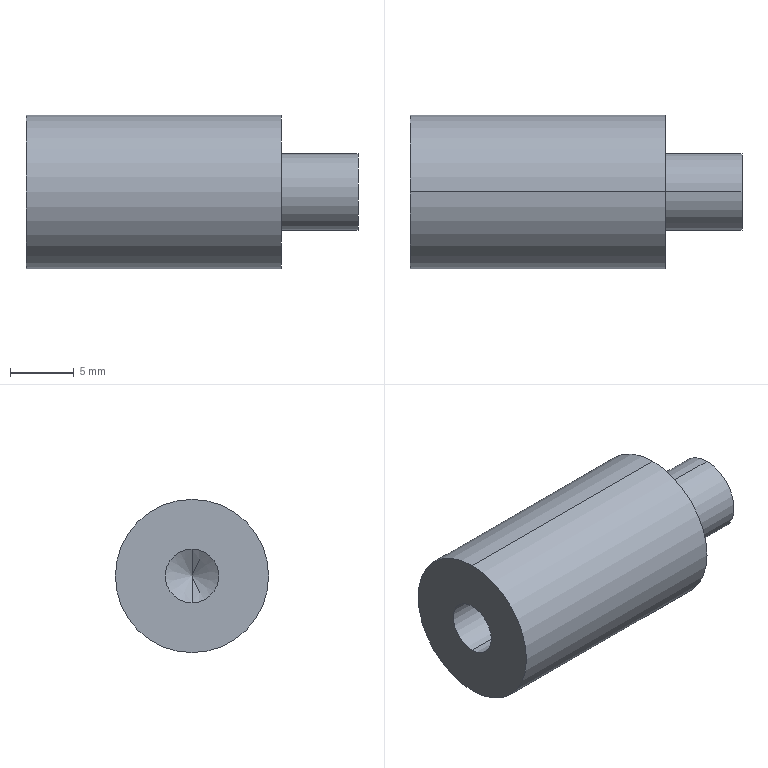Part | STEP file | Tension support column | 1 solid | 15 faces | box 26 x 12 x 12 mm | volume 2216 mm3 | cylinder 8 | cone 4 | plane 3 | commonest cylinder face diameters 2.5 x2 4.2 x2 6 x2 12 x2
STEP:
#1=CARTESIAN_POINT('',(12.4,0.,-2.1));
#2=VERTEX_POINT('',#1);
#3=CARTESIAN_POINT('',(12.4,0.,2.1));
#4=VERTEX_POINT('',#3);
#5=CARTESIAN_POINT('',(12.4,0.,0.));
#6=DIRECTION('',(-1.,0.,0.));
#7=DIRECTION('',(0.,0.,1.));
#8=AXIS2_PLACEMENT_3D('',#5,#6,#7);
#9=CIRCLE('',#8,2.1);
#10=EDGE_CURVE('',#2,#4,#9,.T.);
#11=ORIENTED_EDGE('',*,*,#10,.F.);
#12=CARTESIAN_POINT('',(0.,0.,-2.1));
#13=VERTEX_POINT('',#12);
#14=CARTESIAN_POINT('',(0.,0.,-2.1));
#15=DIRECTION('',(-1.,0.,0.));
#16=VECTOR('',#15,1000.);
#17=LINE('',#14,#16);
#18=EDGE_CURVE('',#2,#13,#17,.T.);
#19=ORIENTED_EDGE('',*,*,#18,.T.);
#20=CARTESIAN_POINT('',(0.,0.,2.1));
#21=VERTEX_POINT('',#20);
#22=CARTESIAN_POINT('',(0.,0.,0.));
#23=DIRECTION('',(-1.,0.,0.));
#24=DIRECTION('',(0.,0.,1.));
#25=AXIS2_PLACEMENT_3D('',#22,#23,#24);
#26=CIRCLE('',#25,2.1);
#27=EDGE_CURVE('',#13,#21,#26,.T.);
#28=ORIENTED_EDGE('',*,*,#27,.T.);
#29=CARTESIAN_POINT('',(0.,0.,2.1));
#30=DIRECTION('',(-1.,0.,0.));
#31=VECTOR('',#30,1000.);
#32=LINE('',#29,#31);
#33=EDGE_CURVE('',#4,#21,#32,.T.);
#34=ORIENTED_EDGE('',*,*,#33,.F.);
#35=EDGE_LOOP('',(#11,#19,#28,#34));
#36=FACE_OUTER_BOUND('',#35,.T.);
#37=CARTESIAN_POINT('',(0.,0.,0.));
#38=DIRECTION('',(-1.,0.,0.));
#39=DIRECTION('',(0.,0.,1.));
#40=AXIS2_PLACEMENT_3D('',#37,#38,#39);
#41=CYLINDRICAL_SURFACE('',#40,2.1);
#42=ADVANCED_FACE('',(#36),#41,.F.);
#43=CARTESIAN_POINT('',(13.662,0.,0.));
#44=VERTEX_POINT('',#43);
#45=CARTESIAN_POINT('',(12.4,0.,2.1));
#46=DIRECTION('',(-0.515,0.,0.8572));
#47=VECTOR('',#46,1000.);
#48=LINE('',#45,#47);
#49=EDGE_CURVE('',#44,#4,#48,.T.);
#50=ORIENTED_EDGE('',*,*,#49,.F.);
#51=CARTESIAN_POINT('',(12.4,0.,-2.1));
#52=DIRECTION('',(-0.515,0.,-0.8572));
#53=VECTOR('',#52,1000.);
#54=LINE('',#51,#53);
#55=EDGE_CURVE('',#44,#2,#54,.T.);
#56=ORIENTED_EDGE('',*,*,#55,.T.);
#57=ORIENTED_EDGE('',*,*,#10,.T.);
#58=EDGE_LOOP('',(#50,#56,#57));
#59=FACE_OUTER_BOUND('',#58,.T.);
#60=CARTESIAN_POINT('',(12.4,0.,0.));
#61=DIRECTION('',(-1.,0.,0.));
#62=DIRECTION('',(0.,0.,1.));
#63=AXIS2_PLACEMENT_3D('',#60,#61,#62);
#64=CONICAL_SURFACE('',#63,2.1,1.03);
#65=ADVANCED_FACE('',(#59),#64,.F.);
#66=CARTESIAN_POINT('',(18.5,0.,1.25));
#67=VERTEX_POINT('',#66);
#68=CARTESIAN_POINT('',(18.5,0.,-1.25));
#69=VERTEX_POINT('',#68);
#70=CARTESIAN_POINT('',(18.5,0.,0.));
#71=DIRECTION('',(1.,0.,0.));
#72=DIRECTION('',(0.,0.,-1.));
#73=AXIS2_PLACEMENT_3D('',#70,#71,#72);
#74=CIRCLE('',#73,1.25);
#75=EDGE_CURVE('',#67,#69,#74,.T.);
#76=ORIENTED_EDGE('',*,*,#75,.F.);
#77=CARTESIAN_POINT('',(26.,0.,1.25));
#78=VERTEX_POINT('',#77);
#79=CARTESIAN_POINT('',(26.,0.,1.25));
#80=DIRECTION('',(1.,0.,0.));
#81=VECTOR('',#80,1000.);
#82=LINE('',#79,#81);
#83=EDGE_CURVE('',#67,#78,#82,.T.);
#84=ORIENTED_EDGE('',*,*,#83,.T.);
#85=CARTESIAN_POINT('',(26.,0.,-1.25));
#86=VERTEX_POINT('',#85);
#87=CARTESIAN_POINT('',(26.,0.,0.));
#88=DIRECTION('',(1.,0.,0.));
#89=DIRECTION('',(0.,0.,-1.));
#90=AXIS2_PLACEMENT_3D('',#87,#88,#89);
#91=CIRCLE('',#90,1.25);
#92=EDGE_CURVE('',#78,#86,#91,.T.);
#93=ORIENTED_EDGE('',*,*,#92,.T.);
#94=CARTESIAN_POINT('',(26.,0.,-1.25));
#95=DIRECTION('',(1.,0.,0.));
#96=VECTOR('',#95,1000.);
#97=LINE('',#94,#96);
#98=EDGE_CURVE('',#69,#86,#97,.T.);
#99=ORIENTED_EDGE('',*,*,#98,.F.);
#100=EDGE_LOOP('',(#76,#84,#93,#99));
#101=FACE_OUTER_BOUND('',#100,.T.);
#102=CARTESIAN_POINT('',(26.,0.,0.));
#103=DIRECTION('',(1.,0.,0.));
#104=DIRECTION('',(0.,0.,-1.));
#105=AXIS2_PLACEMENT_3D('',#102,#103,#104);
#106=CYLINDRICAL_SURFACE('',#105,1.25);
#107=ADVANCED_FACE('',(#101),#106,.F.);
#108=CARTESIAN_POINT('',(17.749,0.,0.));
#109=VERTEX_POINT('',#108);
#110=CARTESIAN_POINT('',(18.5,0.,-1.25));
#111=DIRECTION('',(0.515,0.,-0.8572));
#112=VECTOR('',#111,1000.);
#113=LINE('',#110,#112);
#114=EDGE_CURVE('',#109,#69,#113,.T.);
#115=ORIENTED_EDGE('',*,*,#114,.F.);
#116=CARTESIAN_POINT('',(18.5,0.,1.25));
#117=DIRECTION('',(0.515,0.,0.8572));
#118=VECTOR('',#117,1000.);
#119=LINE('',#116,#118);
#120=EDGE_CURVE('',#109,#67,#119,.T.);
#121=ORIENTED_EDGE('',*,*,#120,.T.);
#122=ORIENTED_EDGE('',*,*,#75,.T.);
#123=EDGE_LOOP('',(#115,#121,#122));
#124=FACE_OUTER_BOUND('',#123,.T.);
#125=CARTESIAN_POINT('',(18.5,0.,0.));
#126=DIRECTION('',(1.,0.,0.));
#127=DIRECTION('',(0.,0.,-1.));
#128=AXIS2_PLACEMENT_3D('',#125,#126,#127);
#129=CONICAL_SURFACE('',#128,1.25,1.03);
#130=ADVANCED_FACE('',(#124),#129,.F.);
#131=CARTESIAN_POINT('',(20.,0.,-3.));
#132=VERTEX_POINT('',#131);
#133=CARTESIAN_POINT('',(20.,0.,3.));
#134=VERTEX_POINT('',#133);
#135=CARTESIAN_POINT('',(20.,0.,0.));
#136=DIRECTION('',(1.,0.,0.));
#137=DIRECTION('',(0.,0.,-1.));
#138=AXIS2_PLACEMENT_3D('',#135,#136,#137);
#139=CIRCLE('',#138,3.);
#140=EDGE_CURVE('',#132,#134,#139,.T.);
#141=ORIENTED_EDGE('',*,*,#140,.T.);
#142=CARTESIAN_POINT('',(26.,0.,3.));
#143=VERTEX_POINT('',#142);
#144=CARTESIAN_POINT('',(0.,0.,3.));
#145=DIRECTION('',(1.,0.,0.));
#146=VECTOR('',#145,1000.);
#147=LINE('',#144,#146);
#148=EDGE_CURVE('',#134,#143,#147,.T.);
#149=ORIENTED_EDGE('',*,*,#148,.T.);
#150=CARTESIAN_POINT('',(26.,0.,-3.));
#151=VERTEX_POINT('',#150);
#152=CARTESIAN_POINT('',(26.,0.,0.));
#153=DIRECTION('',(1.,0.,0.));
#154=DIRECTION('',(0.,0.,-1.));
#155=AXIS2_PLACEMENT_3D('',#152,#153,#154);
#156=CIRCLE('',#155,3.);
#157=EDGE_CURVE('',#151,#143,#156,.T.);
#158=ORIENTED_EDGE('',*,*,#157,.F.);
#159=CARTESIAN_POINT('',(0.,0.,-3.));
#160=DIRECTION('',(1.,0.,0.));
#161=VECTOR('',#160,1000.);
#162=LINE('',#159,#161);
#163=EDGE_CURVE('',#132,#151,#162,.T.);
#164=ORIENTED_EDGE('',*,*,#163,.F.);
#165=EDGE_LOOP('',(#141,#149,#158,#164));
#166=FACE_OUTER_BOUND('',#165,.T.);
#167=CARTESIAN_POINT('',(0.,0.,0.));
#168=DIRECTION('',(1.,0.,0.));
#169=DIRECTION('',(0.,0.,-1.));
#170=AXIS2_PLACEMENT_3D('',#167,#168,#169);
#171=CYLINDRICAL_SURFACE('',#170,3.);
#172=ADVANCED_FACE('',(#166),#171,.T.);
#173=CARTESIAN_POINT('',(0.,0.,-6.));
#174=VERTEX_POINT('',#173);
#175=CARTESIAN_POINT('',(0.,0.,6.));
#176=VERTEX_POINT('',#175);
#177=CARTESIAN_POINT('',(0.,0.,0.));
#178=DIRECTION('',(1.,0.,0.));
#179=DIRECTION('',(0.,0.,-1.));
#180=AXIS2_PLACEMENT_3D('',#177,#178,#179);
#181=CIRCLE('',#180,6.);
#182=EDGE_CURVE('',#174,#176,#181,.T.);
#183=ORIENTED_EDGE('',*,*,#182,.T.);
#184=CARTESIAN_POINT('',(20.,0.,6.));
#185=VERTEX_POINT('',#184);
#186=CARTESIAN_POINT('',(0.,0.,6.));
#187=DIRECTION('',(1.,0.,0.));
#188=VECTOR('',#187,1000.);
#189=LINE('',#186,#188);
#190=EDGE_CURVE('',#176,#185,#189,.T.);
#191=ORIENTED_EDGE('',*,*,#190,.T.);
#192=CARTESIAN_POINT('',(20.,0.,-6.));
#193=VERTEX_POINT('',#192);
#194=CARTESIAN_POINT('',(20.,0.,0.));
#195=DIRECTION('',(1.,0.,0.));
#196=DIRECTION('',(0.,0.,-1.));
#197=AXIS2_PLACEMENT_3D('',#194,#195,#196);
#198=CIRCLE('',#197,6.);
#199=EDGE_CURVE('',#193,#185,#198,.T.);
#200=ORIENTED_EDGE('',*,*,#199,.F.);
#201=CARTESIAN_POINT('',(0.,0.,-6.));
#202=DIRECTION('',(1.,0.,0.));
#203=VECTOR('',#202,1000.);
#204=LINE('',#201,#203);
#205=EDGE_CURVE('',#174,#193,#204,.T.);
#206=ORIENTED_EDGE('',*,*,#205,.F.);
#207=EDGE_LOOP('',(#183,#191,#200,#206));
#208=FACE_OUTER_BOUND('',#207,.T.);
#209=CARTESIAN_POINT('',(0.,0.,0.));
#210=DIRECTION('',(1.,0.,0.));
#211=DIRECTION('',(0.,0.,-1.));
#212=AXIS2_PLACEMENT_3D('',#209,#210,#211);
#213=CYLINDRICAL_SURFACE('',#212,6.);
#214=ADVANCED_FACE('',(#208),#213,.T.);
#215=CARTESIAN_POINT('',(0.,0.,0.));
#216=DIRECTION('',(-1.,0.,0.));
#217=DIRECTION('',(0.,0.,1.));
#218=AXIS2_PLACEMENT_3D('',#215,#216,#217);
#219=CIRCLE('',#218,2.1);
#220=EDGE_CURVE('',#21,#13,#219,.T.);
#221=ORIENTED_EDGE('',*,*,#220,.F.);
#222=ORIENTED_EDGE('',*,*,#27,.F.);
#223=EDGE_LOOP('',(#221,#222));
#224=FACE_BOUND('',#223,.T.);
#225=ORIENTED_EDGE('',*,*,#182,.F.);
#226=CARTESIAN_POINT('',(0.,0.,0.));
#227=DIRECTION('',(1.,0.,0.));
#228=DIRECTION('',(0.,0.,-1.));
#229=AXIS2_PLACEMENT_3D('',#226,#227,#228);
#230=CIRCLE('',#229,6.);
#231=EDGE_CURVE('',#176,#174,#230,.T.);
#232=ORIENTED_EDGE('',*,*,#231,.F.);
#233=EDGE_LOOP('',(#225,#232));
#234=FACE_OUTER_BOUND('',#233,.T.);
#235=CARTESIAN_POINT('',(0.,0.,0.));
#236=DIRECTION('',(-1.,0.,0.));
#237=DIRECTION('',(0.,0.,1.));
#238=AXIS2_PLACEMENT_3D('',#235,#236,#237);
#239=PLANE('',#238);
#240=ADVANCED_FACE('',(#224,#234),#239,.T.);
#241=ORIENTED_EDGE('',*,*,#190,.F.);
#242=ORIENTED_EDGE('',*,*,#231,.T.);
#243=ORIENTED_EDGE('',*,*,#205,.T.);
#244=CARTESIAN_POINT('',(20.,0.,0.));
#245=DIRECTION('',(1.,0.,0.));
#246=DIRECTION('',(0.,0.,-1.));
#247=AXIS2_PLACEMENT_3D('',#244,#245,#246);
#248=CIRCLE('',#247,6.);
#249=EDGE_CURVE('',#185,#193,#248,.T.);
#250=ORIENTED_EDGE('',*,*,#249,.F.);
#251=EDGE_LOOP('',(#241,#242,#243,#250));
#252=FACE_OUTER_BOUND('',#251,.T.);
#253=CARTESIAN_POINT('',(0.,0.,0.));
#254=DIRECTION('',(1.,0.,0.));
#255=DIRECTION('',(0.,0.,-1.));
#256=AXIS2_PLACEMENT_3D('',#253,#254,#255);
#257=CYLINDRICAL_SURFACE('',#256,6.);
#258=ADVANCED_FACE('',(#252),#257,.T.);
#259=ORIENTED_EDGE('',*,*,#199,.T.);
#260=ORIENTED_EDGE('',*,*,#249,.T.);
#261=EDGE_LOOP('',(#259,#260));
#262=FACE_OUTER_BOUND('',#261,.T.);
#263=ORIENTED_EDGE('',*,*,#140,.F.);
#264=CARTESIAN_POINT('',(20.,0.,0.));
#265=DIRECTION('',(1.,0.,0.));
#266=DIRECTION('',(0.,0.,-1.));
#267=AXIS2_PLACEMENT_3D('',#264,#265,#266);
#268=CIRCLE('',#267,3.);
#269=EDGE_CURVE('',#134,#132,#268,.T.);
#270=ORIENTED_EDGE('',*,*,#269,.F.);
#271=EDGE_LOOP('',(#263,#270));
#272=FACE_BOUND('',#271,.T.);
#273=CARTESIAN_POINT('',(20.,6.,0.));
#274=DIRECTION('',(1.,0.,0.));
#275=DIRECTION('',(0.,0.,-1.));
#276=AXIS2_PLACEMENT_3D('',#273,#274,#275);
#277=PLANE('',#276);
#278=ADVANCED_FACE('',(#262,#272),#277,.T.);
#279=ORIENTED_EDGE('',*,*,#148,.F.);
#280=ORIENTED_EDGE('',*,*,#269,.T.);
#281=ORIENTED_EDGE('',*,*,#163,.T.);
#282=CARTESIAN_POINT('',(26.,0.,0.));
#283=DIRECTION('',(1.,0.,0.));
#284=DIRECTION('',(0.,0.,-1.));
#285=AXIS2_PLACEMENT_3D('',#282,#283,#284);
#286=CIRCLE('',#285,3.);
#287=EDGE_CURVE('',#143,#151,#286,.T.);
#288=ORIENTED_EDGE('',*,*,#287,.F.);
#289=EDGE_LOOP('',(#279,#280,#281,#288));
#290=FACE_OUTER_BOUND('',#289,.T.);
#291=CARTESIAN_POINT('',(0.,0.,0.));
#292=DIRECTION('',(1.,0.,0.));
#293=DIRECTION('',(0.,0.,-1.));
#294=AXIS2_PLACEMENT_3D('',#291,#292,#293);
#295=CYLINDRICAL_SURFACE('',#294,3.);
#296=ADVANCED_FACE('',(#290),#295,.T.);
#297=CARTESIAN_POINT('',(26.,0.,0.));
#298=DIRECTION('',(1.,0.,0.));
#299=DIRECTION('',(0.,0.,-1.));
#300=AXIS2_PLACEMENT_3D('',#297,#298,#299);
#301=CIRCLE('',#300,1.25);
#302=EDGE_CURVE('',#86,#78,#301,.T.);
#303=ORIENTED_EDGE('',*,*,#302,.F.);
#304=ORIENTED_EDGE('',*,*,#92,.F.);
#305=EDGE_LOOP('',(#303,#304));
#306=FACE_BOUND('',#305,.T.);
#307=ORIENTED_EDGE('',*,*,#157,.T.);
#308=ORIENTED_EDGE('',*,*,#287,.T.);
#309=EDGE_LOOP('',(#307,#308));
#310=FACE_OUTER_BOUND('',#309,.T.);
#311=CARTESIAN_POINT('',(26.,3.,0.));
#312=DIRECTION('',(1.,0.,0.));
#313=DIRECTION('',(0.,0.,-1.));
#314=AXIS2_PLACEMENT_3D('',#311,#312,#313);
#315=PLANE('',#314);
#316=ADVANCED_FACE('',(#306,#310),#315,.T.);
#317=ORIENTED_EDGE('',*,*,#120,.F.);
#318=ORIENTED_EDGE('',*,*,#114,.T.);
#319=CARTESIAN_POINT('',(18.5,0.,0.));
#320=DIRECTION('',(1.,0.,0.));
#321=DIRECTION('',(0.,0.,-1.));
#322=AXIS2_PLACEMENT_3D('',#319,#320,#321);
#323=CIRCLE('',#322,1.25);
#324=EDGE_CURVE('',#69,#67,#323,.T.);
#325=ORIENTED_EDGE('',*,*,#324,.T.);
#326=EDGE_LOOP('',(#317,#318,#325));
#327=FACE_OUTER_BOUND('',#326,.T.);
#328=CARTESIAN_POINT('',(18.5,0.,0.));
#329=DIRECTION('',(1.,0.,0.));
#330=DIRECTION('',(0.,0.,-1.));
#331=AXIS2_PLACEMENT_3D('',#328,#329,#330);
#332=CONICAL_SURFACE('',#331,1.25,1.03);
#333=ADVANCED_FACE('',(#327),#332,.F.);
#334=ORIENTED_EDGE('',*,*,#83,.F.);
#335=ORIENTED_EDGE('',*,*,#324,.F.);
#336=ORIENTED_EDGE('',*,*,#98,.T.);
#337=ORIENTED_EDGE('',*,*,#302,.T.);
#338=EDGE_LOOP('',(#334,#335,#336,#337));
#339=FACE_OUTER_BOUND('',#338,.T.);
#340=CARTESIAN_POINT('',(26.,0.,0.));
#341=DIRECTION('',(1.,0.,0.));
#342=DIRECTION('',(0.,0.,-1.));
#343=AXIS2_PLACEMENT_3D('',#340,#341,#342);
#344=CYLINDRICAL_SURFACE('',#343,1.25);
#345=ADVANCED_FACE('',(#339),#344,.F.);
#346=ORIENTED_EDGE('',*,*,#55,.F.);
#347=ORIENTED_EDGE('',*,*,#49,.T.);
#348=CARTESIAN_POINT('',(12.4,0.,0.));
#349=DIRECTION('',(-1.,0.,0.));
#350=DIRECTION('',(0.,0.,1.));
#351=AXIS2_PLACEMENT_3D('',#348,#349,#350);
#352=CIRCLE('',#351,2.1);
#353=EDGE_CURVE('',#4,#2,#352,.T.);
#354=ORIENTED_EDGE('',*,*,#353,.T.);
#355=EDGE_LOOP('',(#346,#347,#354));
#356=FACE_OUTER_BOUND('',#355,.T.);
#357=CARTESIAN_POINT('',(12.4,0.,0.));
#358=DIRECTION('',(-1.,0.,0.));
#359=DIRECTION('',(0.,0.,1.));
#360=AXIS2_PLACEMENT_3D('',#357,#358,#359);
#361=CONICAL_SURFACE('',#360,2.1,1.03);
#362=ADVANCED_FACE('',(#356),#361,.F.);
#363=ORIENTED_EDGE('',*,*,#18,.F.);
#364=ORIENTED_EDGE('',*,*,#353,.F.);
#365=ORIENTED_EDGE('',*,*,#33,.T.);
#366=ORIENTED_EDGE('',*,*,#220,.T.);
#367=EDGE_LOOP('',(#363,#364,#365,#366));
#368=FACE_OUTER_BOUND('',#367,.T.);
#369=CARTESIAN_POINT('',(0.,0.,0.));
#370=DIRECTION('',(-1.,0.,0.));
#371=DIRECTION('',(0.,0.,1.));
#372=AXIS2_PLACEMENT_3D('',#369,#370,#371);
#373=CYLINDRICAL_SURFACE('',#372,2.1);
#374=ADVANCED_FACE('',(#368),#373,.F.);
#375=CLOSED_SHELL('',(#42,#65,#107,#130,#172,#214,#240,#258,#278,#296,#316,#333,#345,#362,#374));
#376=MANIFOLD_SOLID_BREP('',#375);
#377=CARTESIAN_POINT('',(0.,0.,0.));
#378=DIRECTION('',(0.,0.,1.));
#379=DIRECTION('',(1.,0.,0.));
#380=AXIS2_PLACEMENT_3D('',#377,#378,#379);
#381=(LENGTH_UNIT()NAMED_UNIT(*)SI_UNIT(.MILLI.,.METRE.));
#382=UNCERTAINTY_MEASURE_WITH_UNIT(LENGTH_MEASURE(0.00001),#381,'','');
#383=(NAMED_UNIT(*)PLANE_ANGLE_UNIT()SI_UNIT($,.RADIAN.));
#384=(NAMED_UNIT(*)SI_UNIT($,.STERADIAN.)SOLID_ANGLE_UNIT());
#385=(GEOMETRIC_REPRESENTATION_CONTEXT(3)GLOBAL_UNCERTAINTY_ASSIGNED_CONTEXT((#382))GLOBAL_UNIT_ASSIGNED_CONTEXT((#381,#383,#384))REPRESENTATION_CONTEXT('',''));
#386=ADVANCED_BREP_SHAPE_REPRESENTATION('',(#376,#380),#385);